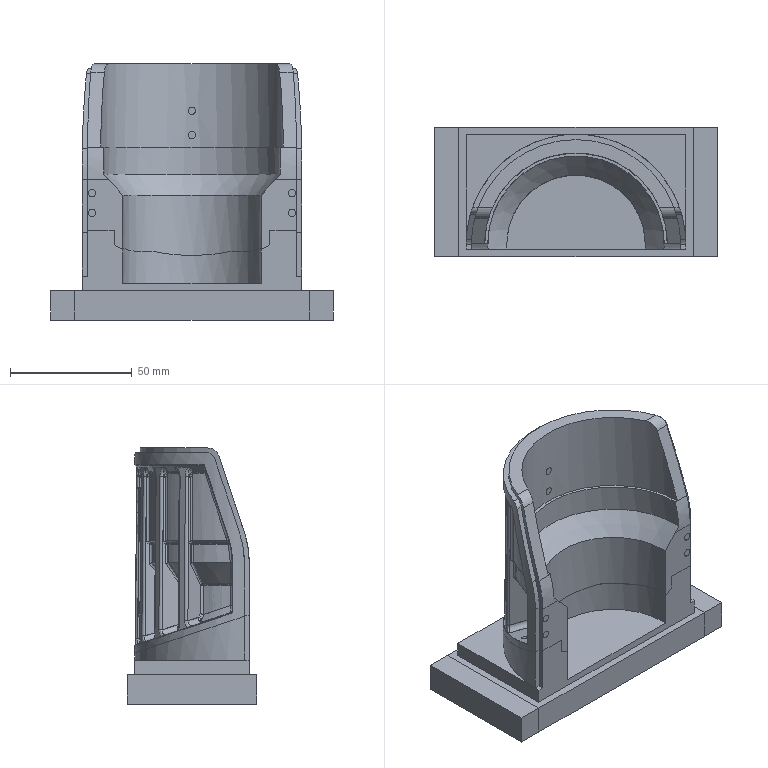NC program | NX | posted by the shop | part box 116 x 53 x 105 mm
Lines 1 to 847 of 44585:
CYCLE800
TRAFOOF
TRANS
ROT
G40 G17 G710 G94 G90 G60 G601 FNORM
TRAFOOF
SUPA G0 Z-1. D0
SUPA G0 X-1.0 Y-1.0
T14 M6
;(T14:C-D8  D=8. R=0.)
;(XY=0.3mm Z=0.3mm)
G54 G90 D1
G0 A0.0 C=DC(0.0)
CYCLE832(0.32,_ROUGH,1.)
G0 X-56.037 Y-1.787 S10000 M3 M8
Z20.3
Z0.0
G94 G1 Z-3. F2500.
X-55.315 Y-1.815
X-54.593 Y-1.795
G3 X-54.008 Y-1.243 I-.195 J.793
X-53.7267 Y2.469 I-70.28 J7.201
G2 X-49.48 Y6.396 I5.1256 J-1.283
X-43.081 Y6.795 I5.081 J-30.011
G1 X49.192 Y6.755
G2 X53.352 Y2.634 I-.936 J-5.104
X53.795 Y-3.659 I-26.663 J-5.04
G1 X53.763 Y-49.155
G2 X49.7756 Y-53.315 I-5.0408 J.841
X43.812 Y-53.793 I-4.878 J23.408
G1 X-49.179 Y-53.76
G2 X-53.322 Y-49.75 I.881 J5.054
X-53.7929 Y-43.811 I23.616 J4.863
G1 X-53.758 Y-1.662
G2 X-53.4017 Y2.116 I18.143 J.192
X-48.353 Y6.206 I5.959 J-2.194
X-40.9 Y6.596 I5.8352 J-40.156
G1 X48.142 Y6.555
G2 X53.058 Y1.922 I-.886 J-5.865
X53.591 Y-4.512 I-25.467 J-5.349
G1 X53.56 Y-48.163
G2 X48.872 Y-53.074 I-5.88 J.92
X42.4103 Y-53.592 I-5.3554 J26.264
G1 X-48.088 Y-53.5678
G2 X-53.0416 Y-48.988 I.816 J5.852
X-53.591 Y-42.581 I24.654 J5.341
G1 X-53.565 Y-2.2076
G2 X-53.06 Y1.852 I12.715 J.48
X-47.675 Y5.974 I6.421 J-2.811
X-40.449 Y6.394 I5.858 J-38.4235
G1 X47.267 Y6.354
G2 X52.824 Y1.249 I-.789 J-6.436
X53.391 Y-5.584 I-27.441 J-5.716
G1 X53.363 Y-47.2383
G2 X48.279 Y-52.818 I-6.43 J.754
X41.322 Y-53.391 I-5.784 J27.669
G1 X-47.277 Y-53.359
G2 X-52.813 Y-48.295 I.7935 J6.425
X-53.39 Y-41.489 I26.879 J5.708
G1 X-53.368 Y-2.632
G2 X-52.586 Y1.907 I10.281 J.566
X-46.832 Y5.801 I6.74 J-3.761
X-38.353 Y6.196 I6.624 J-51.01
G1 X46.517 Y6.151
G2 X52.577 Y.743 I-.691 J-6.873
X53.188 Y-6.236 I-27.558 J-5.931
G1 X53.162 Y-46.46
G2 X47.702 Y-52.59 I-6.888 J.639
X40.547 Y-53.1897 I-6.017 J28.785
G1 X-46.513 Y-53.157
G2 X-52.569 Y-47.775 I.6826 J6.866
X-53.19 Y-40.548 I28.244 J6.065
G1 X-53.159 Y-2.573
G2 X-50.894 Y3.426 I7.822 J.4741
X-44.779 Y5.798 I6.545 J-7.805
X-36.135 Y5.996 I6.885 J-111.823
G1 X45.742 Y5.9555
G2 X52.3612 Y.195 I-.514 J-7.273
X52.99 Y-7.3337 I-30.366 J-6.325
G1 X52.957 Y-45.814
G2 X47.186 Y-52.366 I-7.271 J.587
X39.8073 Y-52.9886 I-6.244 J29.94
G1 X-45.692 Y-52.965
G2 X-52.354 Y-47.229 I.459 J7.269
X-52.988 Y-39.902 I29.262 J6.224
G1 X-52.957 Y-2.833
G2 X-46.61 Y5.187 I7.854 J.306
X-38.876 Y5.788 I6.509 J-33.701
G1 X45.117 Y5.753
G2 X52.15 Y-.316 I-.44 J-7.619
X52.788 Y-7.97 I-31.514 J-6.484
G1 X52.759 Y-45.119
G2 X46.779 Y-52.125 I-7.596 J.428
X39.529 Y-52.784 I-6.287 J28.968
G1 X-45.089 Y-52.7612
G2 X-52.133 Y-46.75 I.402 J7.605
X-52.786 Y-39.324 I29.937 J6.373
G1 X-52.758 Y-3.274
G2 X-46.173 Y4.968 I8.143 J.246
X-38.29 Y5.587 I6.677 J-34.499
G1 X44.493 Y5.553
G2 X51.896 Y-.633 I-.308 J-7.891
X52.585 Y-8.306 I-30.431 J-6.601
G1 X52.557 Y-44.539
G2 X46.288 Y-51.919 I-7.907 J.363
X38.612 Y-52.586 I-6.586 J31.298
G1 X-44.487 Y-52.56
G2 X-51.921 Y-46.282 I.315 J7.913
X-52.585 Y-38.706 I31.007 J6.536
G1 X-52.556 Y-3.682
G2 X-45.755 Y4.751 I8.4005 J.1846
X-37.6484 Y5.387 I6.8726 J-35.631
G1 X43.818 Y5.358
G2 X51.714 Y-1.1845 I-.141 J-8.206
X52.385 Y-9.036 I-32.717 J-6.754
G1 X52.362 Y-43.86
G2 X45.899 Y-51.693 I-8.182 J.169
X38. Y-52.385 I-6.789 J32.066
G1 X-43.814 Y-52.3647
G2 X-51.6994 Y-45.875 I.129 J8.193
X-52.384 Y-38.1 I31.8379 J6.722
G1 X-52.361 Y-4.251
G2 X-48.959 Y2.921 I8.687 J.272
X-42.141 Y5.025 I7.131 J-11.008
X-33.12 Y5.195 I7.598 J-163.607
G1 X43.293 Y5.156
G2 X51.507 Y-1.623 I-.08 J-8.464
X52.184 Y-9.575 I-33.711 J-6.876
G1 X52.156 Y-43.414
G2 X45.453 Y-51.489 I-8.433 J.181
X37.453 Y-52.184 I-6.909 J33.14
G1 X-43.396 Y-52.157
G2 X-51.496 Y-45.423 I.1691 J8.4426
X-52.186 Y-37.223 I34.25 J7.01
G1 X-52.157 Y-4.608
G2 X-47.839 Y3.228 I8.873 J.218
X-44.619 Y4.463 I3.775 J-5.028
X-35.122 Y4.9926 I7.839 J-55.115
G1 X42.7178 Y4.958
G2 X51.267 Y-1.912 I.0639 J-8.674
X51.983 Y-10.085 I-33.712 J-7.074
G1 X51.958 Y-42.835
G2 X44.981 Y-51.296 I-8.692 J.06
X36.905 Y-51.983 I-7.006 J34.553
G1 X-42.864 Y-51.957
G2 X-51.266 Y-45.098 I.07 J8.661
X-51.984 Y-36.825 I34.051 J7.126
G1 X-51.958 Y-5.101
G2 X-48.618 Y2.321 I9.507 J.184
X-44.657 Y4.323 I3.811 J-2.622
X-32.699 Y4.795 I9.718 J-94.462
G1 X42.193 Y4.758
G2 X46.355 Y4.08 I-2.515 J-28.563
X49.206 Y1.683 I-2.44 J-5.7963
X51.605 Y-5.687 I-11.446 J-7.801
X51.7965 Y-14.908 I-148.694 J-7.6967
G1 X51.753 Y-42.414
G2 X44.636 Y-51.075 I-8.89 J.05
X36.161 Y-51.785 I-7.279 J35.99
G1 X-42.238 Y-51.762
G2 X-51.0767 Y-44.63 I-.107 J8.911
X-51.784 Y-36.23 I35.757 J7.242
G1 X-51.757 Y-5.533
G2 X-48.985 Y1.604 I10.614 J-.016
X-44.515 Y4.299 I4.09 J-1.729
X-32.134 Y4.595 I12.048 J-245.243
G1 X41.768 Y4.555
X44.082 Y4.293
X45.232 Y4.293
G3 X45.232 Y6.053 I0. J.88
G1 X28.392 Y6.054
X26.8 Y6.054 Z-2.5
X-26.829 Y6.058 F15000.
X-28.421 Y6.058 Z-3. F2500.
X-44.084 Y6.047
G3 X-43.94 Y4.299 I.145 J-.868
G1 X-30.441 Y4.394
X41.2677 Y4.355
X44.091 Y4.293
G3 X44.091 Y6.053 I0. J.88
G1 X28.392 Y6.054
X26.8 Y6.054 Z-2.5
X-26.83 Y6.058 F15000.
X-28.422 Y6.058 Z-3. F2500.
X-40.884 Y6.047
G3 X-40.74 Y4.299 I.145 J-.868
G2 X-23.054 Y4.195 I4.212 J-784.792
G1 X27.516 Y4.208
X28.624 Y4.299
X42.224 Y4.2937
G3 X42.224 Y6.0537 I0. J.88
G1 X28.358 Y6.043
X26.766 Y6.042 Z-2.5
X-26.6111 Y6.002 F15000.
X-27.241 Y6.008 Z-2.698 F2500.
X-27.87 Y5.976 Z-2.896
X-28.172 Y5.846 Z-3.
G3 X-27.892 Y4.269 I.499 J-.725
X-22.049 Y3.996 I4.428 J32.132
G1 X27.006 Y4.028
X27.51 Y4.206
G3 X27.902 Y5.581 I-.298 J.828
X26.995 Y5.914 Z-2.683 I-.763 J-.676 TURN=0
G1 X26.413 Y5.9147 Z-2.5
X-26.435 Y5.956 F15000.
X-27.066 Y5.964 Z-2.699 F2500.
X-27.697 Y5.933 Z-2.8975
X-27.997 Y5.806 Z-3.
G3 X-27.723 Y4.225 I.494 J-.728
X-22.476 Y3.804 I4.254 J20.1237
G1 X26.43 Y3.829
X27.058 Y4.044
G3 X27.451 Y5.418 I-.298 J.828
X26.544 Y5.752 Z-2.6833 I-.764 J-.675 TURN=0
G1 X25.962 Y5.753 Z-2.5
X-26.029 Y5.819 F15000.
X-26.596 Y5.825 Z-2.6786 F2500.
X-27.163 Y5.7961 Z-2.8572
X-27.375 Y5.716 Z-2.9286
X-27.564 Y5.59 Z-3.
G3 X-27.19 Y4.088 I.593 J-.65
X-22.061 Y3.61 I4.303 J18.4345
G1 X25.832 Y3.627
G3 X26.526 Y3.852 I-.875 J3.884
X26.97 Y5.154 I-.299 J.828
X25.992 Y5.561 Z-2.65 I-.823 J-.6 TURN=0
G1 X25.519 Y5.561 Z-2.5
X-25.618 Y5.628 F15000.
X-26.09 Y5.632 Z-2.649 F2500.
X-26.562 Y5.6 Z-2.798
G3 X-27.08 Y5.241 Z-3. I.225 J-.878 TURN=0
X-26.784 Y3.983 I.731 J-.492
X-22.862 Y3.444 I3.481 J10.783
G1 X-13.685 Y3.393
X25.2851 Y3.4279
G3 X26.315 Y3.751 I-.041 J1.933
X26.613 Y4.921 I-.473 J.744
X25.628 Y5.3752 Z-2.639 I-.84 J-.527 TURN=0
G1 X25.188 Y5.377 Z-2.5
X-25.578 Y5.601 F15000.
X-26.048 Y5.607 Z-2.648 F2500.
X-26.5169 Y5.5756 Z-2.796
G3 X-27.038 Y5.214 Z-3. I.223 J-.878 TURN=0
X-26.741 Y3.958 I.7325 J-.489
X-23.158 Y3.284 I3.335 J7.859
X-13.109 Y3.193 I10.282 J579.266
G1 X24.815 Y3.232
G3 X26.081 Y3.603 I.036 J2.226
X26.38 Y4.772 I-.473 J.744
X25.395 Y5.227 Z-2.639 I-.841 J-.526 TURN=0
G1 X24.956 Y5.23 Z-2.5
X-25.403 Y5.5016 F15000.
X-25.873 Y5.5082 Z-2.648 F2500.
X-26.342 Y5.477 Z-2.796
G3 X-26.863 Y5.116 Z-3. I.222 J-.878 TURN=0
X-26.566 Y3.86 I.732 J-.49
X-23.08 Y3.1144 I3.379 J7.276
X-12.66 Y2.992 I8.731 J300.203
G1 X24.28 Y3.03
G3 X25.805 Y3.4274 I.175 J2.453
X26. Y4.491 I-.588 J.658
X25.014 Y4.967 Z-2.635 I-.847 J-.496 TURN=0
G1 X24.588 Y4.97 Z-2.5
X-25.153 Y5.364 F15000.
X-25.626 Y5.372 Z-2.649 F2500.
X-26.099 Y5.343 Z-2.798
G3 X-26.618 Y4.989 Z-3. I.219 J-.88 TURN=0
X-26.3272 Y3.724 I.7261 J-.499
X-22.554 Y2.916 I3.629 J7.734
X-12.259 Y2.792 I8.834 J305.862
G1 X23.7992 Y2.83
G3 X25.545 Y3.197 I.06 J4.054
G1 X25.713 Y3.346
G3 X25.904 Y4.4206 I-.588 J.658
X24.918 Y4.885 Z-2.637 I-.844 J-.512 TURN=0
G1 X24.485 Y4.888 Z-2.5
X-24.894 Y5.217 F15000.
X-25.367 Y5.224 Z-2.649 F2500.
X-25.839 Y5.195 Z-2.798
G3 X-26.358 Y4.84 Z-3. I.22 J-.88 TURN=0
X-26.066 Y3.576 I.727 J-.497
X-22.378 Y2.74 I3.65 J7.538
X-10.035 Y2.592 I9.353 J265.642
G1 X23.317 Y2.629
G3 X25.365 Y3.037 I.1203 J4.74
G1 X25.552 Y3.203
G3 X25.742 Y4.278 I-.588 J.658
X24.755 Y4.742 Z-2.637 I-.843 J-.513 TURN=0
G1 X24.322 Y4.744 Z-2.5
X-24.544 Y4.992 F15000.
X-25.023 Y5.002 Z-2.651 F2500.
X-25.5009 Y4.961 Z-2.802
G3 X-25.996 Y4.592 Z-3. I.281 J-.893 TURN=0
X-25.806 Y3.429 I.743 J-.475
X-22.24 Y2.566 I3.56 J6.912
X-9.059 Y2.392 I9.6864 J233.999
G1 X22.963 Y2.433
G3 X25.249 Y2.925 I.255 J4.373
G1 X25.375 Y3.045
G3 X25.565 Y4.119 I-.588 J.658
X24.58 Y4.585 Z-2.637 I-.844 J-.511 TURN=0
G1 X24.147 Y4.588 Z-2.5
X-24.507 Y4.959 F15000.
X-24.985 Y4.9698 Z-2.651 F2500.
X-25.461 Y4.93 Z-2.801
G3 X-25.958 Y4.5588 Z-3. I.279 J-.893 TURN=0
X-25.767 Y3.3977 I.744 J-.474
X-22.53 Y2.4353 I3.369 J5.406
X-12.033 Y2.19 I8.187 J125.855
G1 X22.394 Y2.227
G3 X25.1251 Y2.777 I.326 J5.439
G1 X25.289 Y2.965
G3 X25.3647 Y3.942 I-.696 J.546
X24.382 Y4.392 Z-2.641 I-.8395 J-.536 TURN=0
G1 X23.937 Y4.396 Z-2.5
X-24.325 Y4.785 F15000.
X-24.796 Y4.795 Z-2.649 F2500.
X-25.267 Y4.754 Z-2.797
G3 X-25.769 Y4.37 Z-3. I.282 J-.8887 TURN=0
X-25.676 Y3.325 I.754 J-.46
X-22.659 Y2.3 I3.24 J4.583
X-12.829 Y1.991 I7.817 J92.3096
G1 X21.976 Y2.026
G3 X24.999 Y2.622 I.352 J6.178
G1 X25.206 Y2.86
G3 X25.275 Y3.851 I-.696 J.546
X24.296 Y4.288 Z-2.644 I-.836 J-.558 TURN=0
G1 X23.839 Y4.292 Z-2.5
X-24.288 Y4.746 F15000.
X-24.761 Y4.757 Z-2.649 F2500.
X-25.232 Y4.718 Z-2.798
G3 X-25.7338 Y4.3355 Z-3. I.2805 J-.89 TURN=0
X-25.643 Y3.288 I.752 J-.462
X-22.7606 Y2.169 I3.1798 J3.919
X-12.927 Y1.792 I7.834 J75.9706
G1 X21.626 Y1.829
G3 X24.8701 Y2.4632 I.353 J6.803
G1 X25.087 Y2.71
G3 X25.15 Y3.71 I-.695 J.546
X24.174 Y4.137 Z-2.647 I-.833 J-.574 TURN=0
G1 X23.709 Y4.142 Z-2.5
X-24.201 Y4.652 F15000.
X-24.675 Y4.664 Z-2.649 F2500.
X-25.147 Y4.625 Z-2.798
G3 X-25.649 Y4.245 Z-3. I.279 J-.891 TURN=0
X-25.5595 Y3.194 I.75 J-.466
X-22.664 Y2.01 I3.255 J3.826
X-12.7 Y1.593 I7.959 J70.894
G1 X21.119 Y1.624
G3 X24.7 Y2.271 I.389 J8.084
G1 X24.979 Y2.572
G3 X25.041 Y3.573 I-.695 J.546
X24.0655 Y4. Z-2.647 I-.833 J-.5741 TURN=0
G1 X23.6 Y4.005 Z-2.5
X-24.0975 Y4.54 F15000.
X-24.572 Y4.552 Z-2.65 F2500.
X-25.046 Y4.513 Z-2.799
G3 X-25.5467 Y4.1369 Z-3. I.278 J-.892 TURN=0
X-25.46 Y3.082 I.748 J-.469
X-22.493 Y1.837 I3.365 J3.858
X-12.871 Y1.394 I7.837 J65.612
G1 X20.884 Y1.429
G3 X24.577 Y2.113 I.37 J8.324
G1 X24.8423 Y2.399
G3 X24.905 Y3.399 I-.695 J.546
X23.93 Y3.8273 Z-2.647 I-.834 J-.574 TURN=0
G1 X23.4642 Y3.833 Z-2.5
X-23.976 Y4.4081 F15000.
X-24.4524 Y4.421 Z-2.65 F2500.
X-24.927 Y4.383 Z-2.8
G3 X-25.428 Y4.01 Z-3. I.276 J-.893 TURN=0
X-25.343 Y2.952 I.745 J-.473
X-22.382 Y1.673 I3.426 J3.866
X-12.695 Y1.195 I7.932 J62.386
G1 X20.468 Y1.228
G3 X24.413 Y1.925 I.399 J9.2556
G1 X24.777 Y2.3133
G3 X24.708 Y3.1665 I-.811 J.364
X23.7669 Y3.561 Z-2.664 I-.808 J-.607 TURN=0
G1 X23.248 Y3.569 Z-2.5
X-23.861 Y4.275 F15000.
X-24.336 Y4.289 Z-2.65 F2500.
X-24.81 Y4.253 Z-2.799
G3 X-25.3119 Y3.879 Z-3. I.274 J-.893 TURN=0
X-25.227 Y2.821 I.746 J-.473
X-22.234 Y1.501 I3.494 J3.872
X-12.468 Y.996 I8.037 J60.681
G1 X20.212 Y1.031
G3 X24.2724 Y1.747 I.36 J9.834
X24.756 Y2.268 I-.803 J1.231
X24.681 Y3.13 I-.811 J.364
X23.742 Y3.516 Z-2.666 I-.803 J-.621 TURN=0
G1 X23.217 Y3.522 Z-2.5
X-23.724 Y4.127 F15000.
X-24.2011 Y4.14 Z-2.65 F2500.
X-24.677 Y4.103 Z-2.801
G3 X-25.177 Y3.733 Z-3. I.275 J-.894 TURN=0
X-25.094 Y2.671 I.744 J-.476
X-22.107 Y1.333 I3.541 J3.901
X-12.885 Y.8 I7.805 J55.042
G1 X19.763 Y.828
G3 X24.069 Y1.533 I.372 J11.222
X24.711 Y2.167 I-.597 J1.245
X24.626 Y3.042 I-.81 J.364
X23.691 Y3.415 Z-2.669 I-.797 J-.6423 TURN=0
G1 X23.155 Y3.421 Z-2.5
X-23.587 Y3.979 F15000.
X-24.066 Y3.991 Z-2.651 F2500.
X-24.543 Y3.954 Z-2.802
G3 X-25.041 Y3.587 Z-3. I.2748 J-.895 TURN=0
X-24.961 Y2.522 I.741 J-.48
X-21.864 Y1.14 I3.654 J4.028
X-12.411 Y.6 I7.99 J56.823
G1 X19.403 Y.627
G3 X24.002 Y1.39 I.443 J11.574
X24.65 Y2.034 I-.621 J1.272
X24.554 Y2.926 I-.809 J.364
X23.624 Y3.281 Z-2.673 I-.79 J-.671 TURN=0
G1 X23.074 Y3.288 Z-2.5
X-23.447 Y3.827 F15000.
X-23.928 Y3.84 Z-2.651 F2500.
X-24.407 Y3.803 Z-2.803
G3 X-24.904 Y3.44 Z-3. I.274 J-.896 TURN=0
X-24.828 Y2.373 I.738 J-.484
X-21.779 Y.978 I3.652 J3.953
X-12.134 Y.401 I8.1468 J55.254
G1 X19.057 Y.427
G3 X23.856 Y1.202 I.452 J12.445
X24.594 Y1.912 I-.577 J1.339
X24.486 Y2.819 I-.808 J.364
X23.583 Y3.159 Z-2.684 I-.768 J-.673 TURN=0
G1 X22.999 Y3.165 Z-2.5
X-23.274 Y3.632 F15000.
X-23.748 Y3.641 Z-2.649 F2500.
X-24.222 Y3.613 Z-2.799
G3 X-24.741 Y3.263 Z-3. I.216 J-.881 TURN=0
X-24.782 Y2.321 I.728 J-.504
X-22.074 Y.902 I3.3607 J3.122
X-13.435 Y.216 I7.649 J41.571
G1 X18.616 Y.223
G3 X23.641 Y.98 I.465 J13.9854
X24.528 Y1.767 I-.536 J1.498
X24.419 Y2.676 I-.808 J.3636
X23.518 Y3.014 Z-2.685 I-.768 J-.677 TURN=0
G1 X22.931 Y3.021 Z-2.5
X-23.241 Y3.587 F15000.
X-23.717 Y3.597 Z-2.6502 F2500.
X-24.193 Y3.571 Z-2.8004
G3 X-24.712 Y3.2263 Z-3. I.214 J-.883 TURN=0
X-24.757 Y2.277 I.724 J-.51
X-22.244 Y.811 I3.2266 J2.643
X-14.064 Y.032 I7.443 J34.7995
G1 X17.9846 Y.016
G3 X23.444 Y.767 I.59 J15.913
X24.46 Y1.616 I-.511 J1.644
X24.35 Y2.525 I-.8084 J.3636
X23.45 Y2.863 Z-2.6852 I-.768 J-.677 TURN=0
G1 X22.862 Y2.871 Z-2.5
X-23.161 Y3.478 F15000.
X-23.644 Y3.488 Z-2.652 F2500.
X-24.126 Y3.464 Z-2.804
G3 X-24.639 Y3.1325 Z-3. I.21 J-.887 TURN=0
X-24.695 Y2.1691 I.713 J-.525
X-22.107 Y.637 I3.338 J2.687
X-13.836 Y-.166 I7.55 J34.745
G1 X16.966 Y-.197
G3 X22.99 Y.459 I.7756 J20.885
X24.391 Y1.466 I-.418 J2.059
X24.2821 Y2.374 I-.808 J.3636
X23.382 Y2.713 Z-2.685 I-.769 J-.677 TURN=0
G1 X22.794 Y2.722 Z-2.5
X-23.08 Y3.3687 F15000.
X-23.57 Y3.379 Z-2.654 F2500.
X-24.059 Y3.356 Z-2.808
G3 X-24.565 Y3.038 Z-3. I.207 J-.892 TURN=0
X-24.6323 Y2.061 I.701 J-.5391
X-22.062 Y.489 I3.374 J2.63
X-13.925 Y-.357 I7.5348 J32.908
G1 X-4.034 Y-.411
G3 X19.089 Y-.321 I8.039 J900.83
X23.702 Y.656 I.102 J10.907
X24.328 Y1.326 I-.717 J1.296
X24.218 Y2.235 I-.808 J.3636
X23.317 Y2.574 Z-2.685 I-.768 J-.677 TURN=0
G1 X22.73 Y2.581 Z-2.5
X-22.94 Y3.141 F15000.
X-23.438 Y3.151 Z-2.657 F2500.
X-23.935 Y3.128 Z-2.814
X-24.208 Y3.017 Z-2.907
X-24.433 Y2.825 Z-3.
G3 X-24.568 Y1.948 I.692 J-.555
X-22.001 Y.335 I3.392 J2.548
X-13.892 Y-.551 I7.575 J31.799
G1 X-2.558 Y-.611
G3 X19.045 Y-.507 I7.468 J693.693
X23.648 Y.507 I.036 J10.787
X24.273 Y1.203 I-.6567 J1.22
X24.106 Y1.9714 I-.867 J.214
X23.213 Y2.304 Z-2.688 I-.766 J-.6919 TURN=0
G1 X22.615 Y2.3146 Z-2.5
X-22.9331 Y3.139 F15000.
X-23.432 Y3.1512 Z-2.657 F2500.
X-23.93 Y3.1321 Z-2.814
X-24.203 Y3.023 Z-2.907
X-24.429 Y2.833 Z-3.
G3 X-24.568 Y1.948 I.687 J-.561
X-22.354 Y.322 I3.084 J1.876
X-15.133 Y-.7025 I7.127 J24.28
X-2.509 Y-.811 I11.616 J615.688
X18.638 Y-.715 I7.1298 J759.224
X23.528 Y.318 I.1 J11.613
X24.263 Y1.16 I-.604 J1.268
X24.09 Y1.936 I-.866 J.214
X23.199 Y2.2609 Z-2.69 I-.762 J-.704 TURN=0
G1 X22.595 Y2.271 Z-2.5
X-22.88 Y3.046 F15000.
X-23.385 Y3.058 Z-2.6592 F2500.
X-23.89 Y3.04 Z-2.8184
X-24.158 Y2.935 Z-2.9092
X-24.381 Y2.753 Z-3.
G3 X-24.531 Y1.856 I.676 J-.574
X-22.262 Y.158 I3.177 J1.882
X-15.002 Y-.896 I7.209 J24.127
X-1.883 Y-1.0114 I12.032 J620.97
X18.482 Y-.909 I6.806 J673.466
X23.434 Y.142 I.061 J11.9
X24.236 Y1.057 I-.618 J1.351
X24.051 Y1.8486 I-.865 J.215
X23.167 Y2.158 Z-2.695 I-.753 J-.732 TURN=0
G1 X22.549 Y2.169 Z-2.5
X-22.814 Y2.93 F15000.
X-23.358 Y2.948 Z-2.671 F2500.
X-23.9 Y2.913 Z-2.843
X-24.128 Y2.809 Z-2.921
X-24.322 Y2.652 Z-3.
G3 X-24.485 Y1.739 I.662 J-.589
X-22.155 Y-.0124 I3.28 J1.937
X-14.799 Y-1.0921 I7.324 J24.3005
X-2.359 Y-1.212 I12.063 J608.369
X18.189 Y-1.111 I6.827 J706.017
X23.335 Y-.0379 I.087 J12.458
X24.204 Y.9299 I-.628 J1.438
X24.002 Y1.74 I-.863 J.215
X23.147 Y2.031 Z-2.707 I-.73 J-.744 TURN=0
G1 X22.491 Y2.042 Z-2.5
X-22.758 Y2.813 F15000.
X-23.305 Y2.831 Z-2.672 F2500.
X-23.851 Y2.797 Z-2.845
X-24.076 Y2.696 Z-2.922
X-24.269 Y2.543 Z-3.
G3 X-24.439 Y1.6232 I.655 J-.596
X-22.1 Y-.165 I3.339 J1.943
X-14.597 Y-1.2886 I7.459 J24.1973
X17.757 Y-1.321 I17.087 J916.454
X23.119 Y-.283 I.1 J13.857
X24.191 Y.88 I-.556 J1.589
X23.953 Y1.588 I-.891 J.094
X23.109 Y1.8634 Z-2.712 I-.7197 J-.775 TURN=0
G1 X22.435 Y1.876 Z-2.5
X-22.706 Y2.696 F15000.
X-23.254 Y2.715 Z-2.673 F2500.
X-23.802 Y2.682 Z-2.846
X-24.026 Y2.582 Z-2.923
X-24.219 Y2.431 Z-3.
G3 X-24.392 Y1.507 I.651 J-.6
X-22.047 Y-.318 I3.38 J1.924
X-14.632 Y-1.475 I7.47 J23.543
X17.7169 Y-1.51 I17.071 J833.7497
X23.086 Y-.431 I.043 J13.687
X24.181 Y.791 I-.584 J1.625
X23.931 Y1.5111 I-.89 J.095
X23.094 Y1.774 Z-2.716 I-.711 J-.7988 TURN=0
G1 X22.409 Y1.786 Z-2.5
X-22.65 Y2.5576 F15000.
X-23.199 Y2.576 Z-2.673 F2500.
X-23.747 Y2.542 Z-2.846
X-23.97 Y2.443 Z-2.923
X-24.163 Y2.292 Z-3.
G3 X-24.337 Y1.368 I.65 J-.601
X-21.927 Y-.498 I3.481 J2.007
X-14.251 Y-1.68 I7.673 J24.329
X17.378 Y-1.714 I16.727 J830.0303
X22.922 Y-.648 I.05 J14.6906
X24.168 Y.671 I-.592 J1.807
X23.901 Y1.407 I-.888 J.095
X23.074 Y1.655 Z-2.721 I-.7 J-.832 TURN=0
G1 X22.373 Y1.6666 Z-2.5
X-22.604 Y2.441 F15000.
X-23.153 Y2.459 Z-2.673 F2500.
X-23.701 Y2.426 Z-2.846
X-23.924 Y2.326 Z-2.923
X-24.117 Y2.176 Z-3.
G3 X-24.291 Y1.251 I.65 J-.601
X-21.9268 Y-.633 I3.469 J1.928
X-14.4659 Y-1.857 I7.6118 J23.038
X17.247 Y-1.9085 I17.076 J750.563
X22.895 Y-.796 I.04 J14.695
X24.156 Y.571 I-.612 J1.829
X23.876 Y1.32 I-.887 J.095
X23.056 Y1.554 Z-2.725 I-.689 J-.859 TURN=0
G1 X22.342 Y1.564 Z-2.5
X-22.513 Y2.213 F15000.
X-23.059 Y2.227 Z-2.672 F2500.
X-23.604 Y2.2 Z-2.844
X-23.834 Y2.1091 Z-2.922
X-24.033 Y1.962 Z-3.
G3 X-24.275 Y1.2126 I.641 J-.621
X-22.224 Y-.636 I3.182 J1.469
X-15.347 Y-1.991 I7.316 J19.002
X.091 Y-2.212 I11.858 J287.984
X17.713 Y-2.065 I5.5695 J388.807
X23.103 Y-.813 I-.11 J12.703
X24.139 Y.422 I-.71 J1.648
X23.8494 Y1.1767 I-.886 J.0923
X23.057 Y1.403 Z-2.734 I-.672 J-.854 TURN=0
G1 X22.312 Y1.416 Z-2.5
X-22.513 Y2.213 F15000.
X-23.058 Y2.229 Z-2.672 F2500.
X-23.602 Y2.2033 Z-2.8435
X-23.834 Y2.112 Z-2.922
X-24.034 Y1.965 Z-3.
G3 X-24.275 Y1.2126 I.641 J-.6211
X-22.473 Y-.64 I2.932 J1.048
X-15.821 Y-2.138 I7.208 J16.4978
X.042 Y-2.413 I12.057 J238.023
X17.537 Y-2.262 I5.478 J379.958
X23.005 Y-1.004 I-.148 J13.156
X24.127 Y.316 I-.708 J1.738
X23.834 Y1.076 I-.886 J.095
X23.044 Y1.3 Z-2.736 I-.67 J-.86 TURN=0
G1 X22.2964 Y1.313 Z-2.5
X-22.473 Y2.113 F15000.
X-23.027 Y2.129 Z-2.674 F2500.
X-23.58 Y2.106 Z-2.849
X-23.804 Y2.021 Z-2.924
X-24.001 Y1.883 Z-3.
G3 X-24.26 Y1.1138 I.622 J-.638
X-22.382 Y-.815 I3.058 J1.099
X-15.667 Y-2.331 I7.307 J16.735
X-.11 Y-2.613 I11.916 J228.358
X17.155 Y-2.473 I5.3208 J408.217
X22.8295 Y-1.24 I-.1339 J14.29
X24.103 Y.104 I-.775 J2.01
G1 X24.111 Y.179
G3 X23.815 Y.9428 I-.885 J.096
X23.028 Y1.163 Z-2.737 I-.668 J-.87 TURN=0
G1 X22.275 Y1.177 Z-2.5
X-22.443 Y2.038 F15000.
X-23.003 Y2.054 Z-2.676 F2500.
X-23.562 Y2.034 Z-2.853
X-23.7817 Y1.952 Z-2.926
X-23.976 Y1.822 Z-3.
G3 X-24.248 Y1.0397 I.608 J-.65
X-22.384 Y-.942 I3.074 J1.023
X-15.607 Y-2.5173 I7.3924 J16.442
X.416 Y-2.813 I12.209 J227.315
X17.2542 Y-2.651 I5.148 J340.2897
X22.922 Y-1.325 I-.188 J13.577
X24.103 Y.085 I-.714 J1.798
X23.786 Y.763 I-.896 J-.006
X23.011 Y.9714 Z-2.742 I-.658 J-.901 TURN=0
G1 X22.242 Y.988 Z-2.5
X-22.408 Y1.937 F15000.
X-22.974 Y1.954 Z-2.678 F2500.
X-23.54 Y1.936 Z-2.857
X-23.754 Y1.86 Z-2.928
X-23.946 Y1.737 Z-3.
G3 X-24.233 Y.9409 I.592 J-.663
X-22.404 Y-1.061 I3.095 J.992
X-15.662 Y-2.693 I7.423 J15.92
X.889 Y-3.015 I12.559 J220.396
X17.1248 Y-2.845 I4.809 J316.8
X22.842 Y-1.51 I-.238 J13.9252
X24.102 Y-.104 I-.857 J2.037
G1 X24.103 Y.021
G3 X23.778 Y.7051 I-.895 J-.005
X23.008 Y.907 Z-2.7443 I-.651 J-.913 TURN=0
G1 X22.232 Y.922 Z-2.5
X-22.375 Y1.814 F15000.
X-22.946 Y1.83 Z-2.68 F2500.
X-23.517 Y1.814 Z-2.86
X-23.727 Y1.74 Z-2.93
X-23.916 Y1.622 Z-3.
G3 X-24.214 Y.8174 I.581 J-.673
X-22.317 Y-1.239 I3.211 J1.059
X-15.647 Y-2.875 I7.454 J15.978
X-1.408 Y-3.2147 I11.407 J179.3396
X16.744 Y-3.057 I5.585 J402.121
X22.722 Y-1.718 I-.187 J14.851
X24.102 Y-.225 I-.873 J2.192
G1 X24.102 Y-.1
G3 X23.763 Y.596 I-.894 J-.005
X23.003 Y.7864 Z-2.749 I-.64 J-.944 TURN=0
G1 X22.213 Y.803 Z-2.5
X-22.3474 Y1.715 F15000.
X-22.923 Y1.731 Z-2.681 F2500.
X-23.498 Y1.716 Z-2.862
X-23.7044 Y1.644 Z-2.931
X-23.891 Y1.531 Z-3.
G3 X-24.1983 Y.7186 I.571 J-.68
X-22.308 Y-1.375 I3.2325 J1.018
X-15.518 Y-3.067 I7.574 J15.929
X1.016 Y-3.414 I12.625 J207.046
X16.775 Y-3.24 I4.7059 J287.276
X22.735 Y-1.852 I-.259 J14.601
X24.102 Y-.353 I-.926 J2.218
G1 X24.102 Y-.203
G3 X23.75 Y.503 I-.893 J-.005
X22.942 Y.685 Z-2.735 I-.665 J-1.068 TURN=0
G1 X22.197 Y.7 Z-2.5
X-22.314 Y1.591 F15000.
X-22.894 Y1.607 Z-2.6828 F2500.
X-23.475 Y1.593 Z-2.8656
X-23.677 Y1.524 Z-2.9328
X-23.861 Y1.417 Z-3.
G3 X-24.179 Y.595 I.56 J-.689
X-22.238 Y-1.547 I3.317 J1.055
X-15.481 Y-3.25 I7.621 J15.982
X.839 Y-3.615 I12.566 J196.795
X16.677 Y-3.432 I4.548 J292.292
X22.73 Y-1.997 I-.277 J14.65
X24.102 Y-.4748 I-.964 J2.248
G1 X24.102 Y-.3498
G3 X23.732 Y.3691 I-.891 J-.004
X22.936 Y.538 Z-2.74 I-.653 J-1.117 TURN=0
G1 X22.174 Y.554 Z-2.5
X-22.286 Y1.467 F15000.
X-22.8692 Y1.483 Z-2.684 F2500.
X-23.453 Y1.47 Z-2.867
X-23.652 Y1.403 Z-2.934
X-23.835 Y1.299 Z-3.
G3 X-24.16 Y.472 I.5528 J-.6942
X-22.216 Y-1.693 I3.359 J1.061
X-15.376 Y-3.44 I7.724 J15.976
X-.358 Y-3.815 I11.922 J176.495
X16.312 Y-3.644 I4.903 J334.3849
X22.592 Y-2.22 I-.241 J15.618
X24.101 Y-.607 I-.976 J2.426
G1 X24.102 Y-.457
G3 X23.718 Y.271 I-.89 J-.004
X22.93 Y.431 Z-2.743 I-.644 J-1.155 TURN=0
G1 X22.157 Y.446 Z-2.5
X-22.267 Y1.344 F15000.
X-22.85 Y1.359 Z-2.684 F2500.
X-23.433 Y1.347 Z-2.867
X-23.633 Y1.28 Z-2.934
X-23.816 Y1.175 Z-3.
G3 X-24.14 Y.348 I.553 J-.694
X-22.179 Y-1.849 I3.409 J1.069
X-15.317 Y-3.626 I7.796 J15.967
X-1.08 Y-4.015 I11.568 J162.804
X16.184 Y-3.839 I5.128 J344.764
X22.469 Y-2.433 I-.312 J16.146
X24.098 Y-.77 I-1.048 J2.657
G1 X24.102 Y-.588
G3 X23.707 Y.148 I-.89 J-.003
X22.926 Y.3 Z-2.746 I-.636 J-1.186 TURN=0
G1 X22.144 Y.316 Z-2.5
X-22.247 Y1.22 F15000.
X-22.831 Y1.236 Z-2.684 F2500.
X-23.414 Y1.223 Z-2.867
X-23.614 Y1.156 Z-2.934
X-23.7965 Y1.051 Z-3.
G3 X-24.121 Y.225 I.553 J-.694
X-22.205 Y-1.969 I3.4085 J1.043
X-15.486 Y-3.7878 I7.769 J15.385
X-1.977 Y-4.213 I11.258 J142.7306
X15.94 Y-4.043 I5.445 J368.6
X22.423 Y-2.605 I-.2821 J16.611
X24.098 Y-.9016 I-1.084 J2.742
G1 X24.101 Y-.718
G3 X23.698 Y.024 I-.889 J-.003
X22.921 Y.169 Z-2.748 I-.629 J-1.208 TURN=0
G1 X22.133 Y.1831 Z-2.5
X-22.208 Y.966 F15000.
X-22.7954 Y.979 Z-2.6851 F2500.
X-23.3833 Y.967 Z-2.87
X-23.579 Y.901 Z-2.9351
X-23.7589 Y.8009 Z-3.
G3 X-24.102 Y.104 I.55 J-.704
X-22.247 Y-2.079 I3.3687 J.982
X-15.472 Y-3.968 I7.845 J15.045
X.018 Y-4.416 I12.325 J158.206
X16.182 Y-4.211 I4.592 J274.966
X22.53 Y-2.694 I-.406 J15.742
X24.101 Y-1.0026 I-1.07 J2.5682
G1 X24.101 Y-.847
G3 X23.693 Y-.103 I-.889 J-.003
X22.921 Y.041 Z-2.75 I-.628 J-1.227 TURN=0
G1 X22.127 Y.057 Z-2.5
X-22.208 Y.966 F15000.
X-22.795 Y.981 Z-2.685 F2500.
X-23.382 Y.97 Z-2.87
X-23.578 Y.9045 Z-2.935
X-23.759 Y.804 Z-3.
G3 X-24.102 Y.104 I.55 J-.704
X-22.486 Y-2.06 I3.079 J.614
X-16.09 Y-4.07 I7.65 J13.167
X-2.597 Y-4.611 I11.384 J115.324
X15.662 Y-4.435 I5.653 J360.87
X22.315 Y-2.961 I-.334 J17.261
X24.0946 Y-1.191 I-1.154 J2.939
G1 X24.101 Y-.997
G3 X23.6915 Y-.255 I-.889 J-.006
X22.943 Y-.112 Z-2.757 I-.614 J-1.186 TURN=0
G1 X22.126 Y-.094 Z-2.5
X-22.196 Y.889 F15000.
X-22.808 Y.9104 Z-2.693 F2500.
X-23.42 Y.886 Z-2.886
X-23.59 Y.822 Z-2.943
X-23.749 Y.736 Z-3.
G3 X-24.102 Y.029 I.54 J-.711
X-22.5424 Y-2.155 I3.0597 J.536
X-16.121 Y-4.241 I7.704 J12.786
X-2.1224 Y-4.812 I11.699 J115.042
X15.349 Y-4.643 I5.257 J360.825
X22.195 Y-3.175 I-.308 J18.124
X24.09 Y-1.3514 I-1.201 J3.143
G1 X24.098 Y-1.151
G3 X23.69 Y-.393 I-.889 J.011
X22.9203 Y-.248 Z-2.75 I-.629 J-1.231 TURN=0
G1 X22.125 Y-.23 Z-2.5
X-22.1794 Y.787 F15000.
X-22.796 Y.81 Z-2.694 F2500.
X-23.413 Y.7872 Z-2.889
X-23.736 Y.645 Z-3.
G3 X-24.102 Y-.071 I.526 J-.72
X-22.5708 Y-2.269 I3.085 J.5159
X-16.2186 Y-4.403 I7.715 J12.447
X-2.296 Y-5.011 I11.72 J108.698
X15.314 Y-4.833 I5.34 J343.647
X22.167 Y-3.341 I-.37 J18.184
X24.086 Y-1.5062 I-1.256 J3.233
G1 X24.096 Y-1.296
G3 X23.689 Y-.539 I-.889 J.011
X22.919 Y-.3935 Z-2.75 I-.631 J-1.23 TURN=0
G1 X22.123 Y-.374 Z-2.5
X-22.164 Y.686 F15000.
X-22.785 Y.709 Z-2.696 F2500.
X-23.407 Y.689 Z-2.892
X-23.723 Y.554 Z-3.
G3 X-24.1018 Y-.171 I.512 J-.729
X-22.571 Y-2.405 I3.119 J.495
X-16.249 Y-4.573 I7.753 J12.302
X-2.965 Y-5.207 I11.445 J100.38
X15.048 Y-5.038 I5.759 J347.559